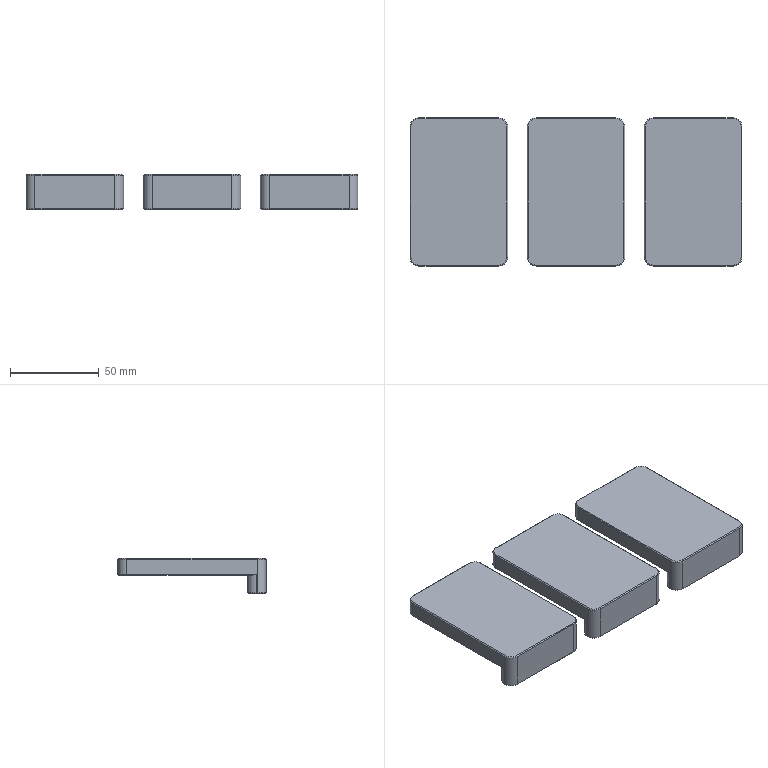NC program | NX | posted with a generic post | part box 187 x 83.5 x 20 mm
Lines 21 to 832 of 5666:
(ZLEVEL_PROFILE_COPY_1 , TOOL : D10)
N40 T15 M6
N42 G54
N44 G17 G0 G90 X-93.244 Y-45.694 S9500 M3
N46 G43 Z30. H15
N48 Z1.5
N50 G94 G1 X-94.903 Y-44.6 Z1.396 F1000.
N52 X-96.35 Y-43.153 Z1.289
N54 X-97.477 Y-41.444 Z1.181
N56 X-98.237 Y-39.543 Z1.074
N58 X-98.6 Y-37.529 Z0.967
N60 Y0. Z-1.
N62 Y36.75 F3500.
N64 G2 X-88.5 Y46.85 R10.1
N66 G1 X-43.5
N68 G2 X-33.4 Y36.75 R10.1
N70 G1 Y-36.75
N72 G2 X-43.5 Y-46.85 R10.1
N74 G1 X-88.5
N76 G2 X-98.6 Y-36.75 R10.1
N78 G1 Y0.
N80 Y36.75 Z-1.122
N82 X-98.574 Y37.471 Z-1.125
N84 X-98.497 Y38.187 Z-1.127
N86 X-98.369 Y38.897 Z-1.13
N88 X-98.191 Y39.595 Z-1.132
N90 X-97.963 Y40.28 Z-1.134
N92 X-97.687 Y40.946 Z-1.137
N94 X-97.365 Y41.59 Z-1.139
N96 X-96.997 Y42.21 Z-1.142
N98 X-96.585 Y42.803 Z-1.144
N100 X-96.133 Y43.364 Z-1.146
N102 X-95.642 Y43.892 Z-1.149
N104 X-95.114 Y44.383 Z-1.151
N106 X-94.553 Y44.835 Z-1.154
N108 X-93.96 Y45.247 Z-1.156
N110 X-93.34 Y45.615 Z-1.158
N112 X-92.696 Y45.937 Z-1.161
N114 X-92.03 Y46.213 Z-1.163
N116 X-91.345 Y46.441 Z-1.166
N118 X-90.647 Y46.619 Z-1.168
N120 X-89.937 Y46.747 Z-1.17
N122 X-89.221 Y46.824 Z-1.173
N124 X-88.5 Y46.85 Z-1.175
N126 X-43.5 Z-1.325
N128 X-42.779 Y46.824 Z-1.327
N130 X-42.063 Y46.747 Z-1.33
N132 X-41.353 Y46.619 Z-1.332
N134 X-40.655 Y46.441 Z-1.334
N136 X-39.97 Y46.213 Z-1.337
N138 X-39.304 Y45.937 Z-1.339
N140 X-38.66 Y45.615 Z-1.342
N142 X-38.04 Y45.247 Z-1.344
N144 X-37.447 Y44.835 Z-1.346
N146 X-36.886 Y44.383 Z-1.349
N148 X-36.358 Y43.892 Z-1.351
N150 X-35.867 Y43.364 Z-1.354
N152 X-35.415 Y42.803 Z-1.356
N154 X-35.003 Y42.21 Z-1.358
N156 X-34.635 Y41.59 Z-1.361
N158 X-34.313 Y40.946 Z-1.363
N160 X-34.037 Y40.28 Z-1.366
N162 X-33.809 Y39.595 Z-1.368
N164 X-33.631 Y38.897 Z-1.37
N166 X-33.503 Y38.187 Z-1.373
N168 X-33.426 Y37.471 Z-1.375
N170 X-33.4 Y36.75 Z-1.378
N172 Y-36.75 Z-1.622
N174 X-33.426 Y-37.471 Z-1.625
N176 X-33.503 Y-38.187 Z-1.627
N178 X-33.631 Y-38.897 Z-1.63
N180 X-33.809 Y-39.595 Z-1.632
N182 X-34.037 Y-40.28 Z-1.634
N184 X-34.313 Y-40.946 Z-1.637
N186 X-34.635 Y-41.59 Z-1.639
N188 X-35.003 Y-42.21 Z-1.642
N190 X-35.415 Y-42.803 Z-1.644
N192 X-35.867 Y-43.364 Z-1.646
N194 X-36.358 Y-43.892 Z-1.649
N196 X-36.886 Y-44.383 Z-1.651
N198 X-37.447 Y-44.835 Z-1.654
N200 X-38.04 Y-45.247 Z-1.656
N202 X-38.66 Y-45.615 Z-1.658
N204 X-39.304 Y-45.937 Z-1.661
N206 X-39.97 Y-46.213 Z-1.663
N208 X-40.655 Y-46.441 Z-1.666
N210 X-41.353 Y-46.619 Z-1.668
N212 X-42.063 Y-46.747 Z-1.67
N214 X-42.779 Y-46.824 Z-1.673
N216 X-43.5 Y-46.85 Z-1.675
N218 X-88.5 Z-1.825
N220 X-89.221 Y-46.824 Z-1.827
N222 X-89.937 Y-46.747 Z-1.83
N224 X-90.647 Y-46.619 Z-1.832
N226 X-91.345 Y-46.441 Z-1.834
N228 X-92.03 Y-46.213 Z-1.837
N230 X-92.696 Y-45.937 Z-1.839
N232 X-93.34 Y-45.615 Z-1.842
N234 X-93.96 Y-45.247 Z-1.844
N236 X-94.553 Y-44.835 Z-1.846
N238 X-95.114 Y-44.383 Z-1.849
N240 X-95.642 Y-43.892 Z-1.851
N242 X-96.133 Y-43.364 Z-1.854
N244 X-96.585 Y-42.803 Z-1.856
N246 X-96.997 Y-42.21 Z-1.858
N248 X-97.365 Y-41.59 Z-1.861
N250 X-97.687 Y-40.946 Z-1.863
N252 X-97.963 Y-40.28 Z-1.866
N254 X-98.191 Y-39.595 Z-1.868
N256 X-98.369 Y-38.897 Z-1.87
N258 X-98.497 Y-38.187 Z-1.873
N260 X-98.574 Y-37.471 Z-1.875
N262 X-98.6 Y-36.75 Z-1.878
N264 Y0. Z-2.
N266 Y36.75 Z-2.122
N268 X-98.574 Y37.471 Z-2.125
N270 X-98.497 Y38.187 Z-2.127
N272 X-98.369 Y38.897 Z-2.13
N274 X-98.191 Y39.595 Z-2.132
N276 X-97.963 Y40.28 Z-2.134
N278 X-97.687 Y40.946 Z-2.137
N280 X-97.365 Y41.59 Z-2.139
N282 X-96.997 Y42.21 Z-2.142
N284 X-96.585 Y42.803 Z-2.144
N286 X-96.133 Y43.364 Z-2.146
N288 X-95.642 Y43.892 Z-2.149
N290 X-95.114 Y44.383 Z-2.151
N292 X-94.553 Y44.835 Z-2.154
N294 X-93.96 Y45.247 Z-2.156
N296 X-93.34 Y45.615 Z-2.158
N298 X-92.696 Y45.937 Z-2.161
N300 X-92.03 Y46.213 Z-2.163
N302 X-91.345 Y46.441 Z-2.166
N304 X-90.647 Y46.619 Z-2.168
N306 X-89.937 Y46.747 Z-2.17
N308 X-89.221 Y46.824 Z-2.173
N310 X-88.5 Y46.85 Z-2.175
N312 X-43.5 Z-2.325
N314 X-42.779 Y46.824 Z-2.327
N316 X-42.063 Y46.747 Z-2.33
N318 X-41.353 Y46.619 Z-2.332
N320 X-40.655 Y46.441 Z-2.334
N322 X-39.97 Y46.213 Z-2.337
N324 X-39.304 Y45.937 Z-2.339
N326 X-38.66 Y45.615 Z-2.342
N328 X-38.04 Y45.247 Z-2.344
N330 X-37.447 Y44.835 Z-2.346
N332 X-36.886 Y44.383 Z-2.349
N334 X-36.358 Y43.892 Z-2.351
N336 X-35.867 Y43.364 Z-2.354
N338 X-35.415 Y42.803 Z-2.356
N340 X-35.003 Y42.21 Z-2.358
N342 X-34.635 Y41.59 Z-2.361
N344 X-34.313 Y40.946 Z-2.363
N346 X-34.037 Y40.28 Z-2.366
N348 X-33.809 Y39.595 Z-2.368
N350 X-33.631 Y38.897 Z-2.37
N352 X-33.503 Y38.187 Z-2.373
N354 X-33.426 Y37.471 Z-2.375
N356 X-33.4 Y36.75 Z-2.378
N358 Y-36.75 Z-2.622
N360 X-33.426 Y-37.471 Z-2.625
N362 X-33.503 Y-38.187 Z-2.627
N364 X-33.631 Y-38.897 Z-2.63
N366 X-33.809 Y-39.595 Z-2.632
N368 X-34.037 Y-40.28 Z-2.634
N370 X-34.313 Y-40.946 Z-2.637
N372 X-34.635 Y-41.59 Z-2.639
N374 X-35.003 Y-42.21 Z-2.642
N376 X-35.415 Y-42.803 Z-2.644
N378 X-35.867 Y-43.364 Z-2.646
N380 X-36.358 Y-43.892 Z-2.649
N382 X-36.886 Y-44.383 Z-2.651
N384 X-37.447 Y-44.835 Z-2.654
N386 X-38.04 Y-45.247 Z-2.656
N388 X-38.66 Y-45.615 Z-2.658
N390 X-39.304 Y-45.937 Z-2.661
N392 X-39.97 Y-46.213 Z-2.663
N394 X-40.655 Y-46.441 Z-2.666
N396 X-41.353 Y-46.619 Z-2.668
N398 X-42.063 Y-46.747 Z-2.67
N400 X-42.779 Y-46.824 Z-2.673
N402 X-43.5 Y-46.85 Z-2.675
N404 X-88.5 Z-2.825
N406 X-89.221 Y-46.824 Z-2.827
N408 X-89.937 Y-46.747 Z-2.83
N410 X-90.647 Y-46.619 Z-2.832
N412 X-91.345 Y-46.441 Z-2.834
N414 X-92.03 Y-46.213 Z-2.837
N416 X-92.696 Y-45.937 Z-2.839
N418 X-93.34 Y-45.615 Z-2.842
N420 X-93.96 Y-45.247 Z-2.844
N422 X-94.553 Y-44.835 Z-2.846
N424 X-95.114 Y-44.383 Z-2.849
N426 X-95.642 Y-43.892 Z-2.851
N428 X-96.133 Y-43.364 Z-2.854
N430 X-96.585 Y-42.803 Z-2.856
N432 X-96.997 Y-42.21 Z-2.858
N434 X-97.365 Y-41.59 Z-2.861
N436 X-97.687 Y-40.946 Z-2.863
N438 X-97.963 Y-40.28 Z-2.866
N440 X-98.191 Y-39.595 Z-2.868
N442 X-98.369 Y-38.897 Z-2.87
N444 X-98.497 Y-38.187 Z-2.873
N446 X-98.574 Y-37.471 Z-2.875
N448 X-98.6 Y-36.75 Z-2.878
N450 Y0. Z-3.
N452 Y36.75 Z-3.122
N454 X-98.574 Y37.471 Z-3.125
N456 X-98.497 Y38.187 Z-3.127
N458 X-98.369 Y38.897 Z-3.13
N460 X-98.191 Y39.595 Z-3.132
N462 X-97.963 Y40.28 Z-3.134
N464 X-97.687 Y40.946 Z-3.137
N466 X-97.365 Y41.59 Z-3.139
N468 X-96.997 Y42.21 Z-3.142
N470 X-96.585 Y42.803 Z-3.144
N472 X-96.133 Y43.364 Z-3.146
N474 X-95.642 Y43.892 Z-3.149
N476 X-95.114 Y44.383 Z-3.151
N478 X-94.553 Y44.835 Z-3.154
N480 X-93.96 Y45.247 Z-3.156
N482 X-93.34 Y45.615 Z-3.158
N484 X-92.696 Y45.937 Z-3.161
N486 X-92.03 Y46.213 Z-3.163
N488 X-91.345 Y46.441 Z-3.166
N490 X-90.647 Y46.619 Z-3.168
N492 X-89.937 Y46.747 Z-3.17
N494 X-89.221 Y46.824 Z-3.173
N496 X-88.5 Y46.85 Z-3.175
N498 X-43.5 Z-3.325
N500 X-42.779 Y46.824 Z-3.327
N502 X-42.063 Y46.747 Z-3.33
N504 X-41.353 Y46.619 Z-3.332
N506 X-40.655 Y46.441 Z-3.334
N508 X-39.97 Y46.213 Z-3.337
N510 X-39.304 Y45.937 Z-3.339
N512 X-38.66 Y45.615 Z-3.342
N514 X-38.04 Y45.247 Z-3.344
N516 X-37.447 Y44.835 Z-3.346
N518 X-36.886 Y44.383 Z-3.349
N520 X-36.358 Y43.892 Z-3.351
N522 X-35.867 Y43.364 Z-3.354
N524 X-35.415 Y42.803 Z-3.356
N526 X-35.003 Y42.21 Z-3.358
N528 X-34.635 Y41.59 Z-3.361
N530 X-34.313 Y40.946 Z-3.363
N532 X-34.037 Y40.28 Z-3.366
N534 X-33.809 Y39.595 Z-3.368
N536 X-33.631 Y38.897 Z-3.37
N538 X-33.503 Y38.187 Z-3.373
N540 X-33.426 Y37.471 Z-3.375
N542 X-33.4 Y36.75 Z-3.378
N544 Y-36.75 Z-3.622
N546 X-33.426 Y-37.471 Z-3.625
N548 X-33.503 Y-38.187 Z-3.627
N550 X-33.631 Y-38.897 Z-3.63
N552 X-33.809 Y-39.595 Z-3.632
N554 X-34.037 Y-40.28 Z-3.634
N556 X-34.313 Y-40.946 Z-3.637
N558 X-34.635 Y-41.59 Z-3.639
N560 X-35.003 Y-42.21 Z-3.642
N562 X-35.415 Y-42.803 Z-3.644
N564 X-35.867 Y-43.364 Z-3.646
N566 X-36.358 Y-43.892 Z-3.649
N568 X-36.886 Y-44.383 Z-3.651
N570 X-37.447 Y-44.835 Z-3.654
N572 X-38.04 Y-45.247 Z-3.656
N574 X-38.66 Y-45.615 Z-3.658
N576 X-39.304 Y-45.937 Z-3.661
N578 X-39.97 Y-46.213 Z-3.663
N580 X-40.655 Y-46.441 Z-3.666
N582 X-41.353 Y-46.619 Z-3.668
N584 X-42.063 Y-46.747 Z-3.67
N586 X-42.779 Y-46.824 Z-3.673
N588 X-43.5 Y-46.85 Z-3.675
N590 X-88.5 Z-3.825
N592 X-89.221 Y-46.824 Z-3.827
N594 X-89.937 Y-46.747 Z-3.83
N596 X-90.647 Y-46.619 Z-3.832
N598 X-91.345 Y-46.441 Z-3.834
N600 X-92.03 Y-46.213 Z-3.837
N602 X-92.696 Y-45.937 Z-3.839
N604 X-93.34 Y-45.615 Z-3.842
N606 X-93.96 Y-45.247 Z-3.844
N608 X-94.553 Y-44.835 Z-3.846
N610 X-95.114 Y-44.383 Z-3.849
N612 X-95.642 Y-43.892 Z-3.851
N614 X-96.133 Y-43.364 Z-3.854
N616 X-96.585 Y-42.803 Z-3.856
N618 X-96.997 Y-42.21 Z-3.858
N620 X-97.365 Y-41.59 Z-3.861
N622 X-97.687 Y-40.946 Z-3.863
N624 X-97.963 Y-40.28 Z-3.866
N626 X-98.191 Y-39.595 Z-3.868
N628 X-98.369 Y-38.897 Z-3.87
N630 X-98.497 Y-38.187 Z-3.873
N632 X-98.574 Y-37.471 Z-3.875
N634 X-98.6 Y-36.75 Z-3.878
N636 Y0. Z-4.
N638 Y36.75 Z-4.122
N640 X-98.574 Y37.471 Z-4.125
N642 X-98.497 Y38.187 Z-4.127
N644 X-98.369 Y38.897 Z-4.13
N646 X-98.191 Y39.595 Z-4.132
N648 X-97.963 Y40.28 Z-4.134
N650 X-97.687 Y40.946 Z-4.137
N652 X-97.365 Y41.59 Z-4.139
N654 X-96.997 Y42.21 Z-4.142
N656 X-96.585 Y42.803 Z-4.144
N658 X-96.133 Y43.364 Z-4.146
N660 X-95.642 Y43.892 Z-4.149
N662 X-95.114 Y44.383 Z-4.151
N664 X-94.553 Y44.835 Z-4.154
N666 X-93.96 Y45.247 Z-4.156
N668 X-93.34 Y45.615 Z-4.158
N670 X-92.696 Y45.937 Z-4.161
N672 X-92.03 Y46.213 Z-4.163
N674 X-91.345 Y46.441 Z-4.166
N676 X-90.647 Y46.619 Z-4.168
N678 X-89.937 Y46.747 Z-4.17
N680 X-89.221 Y46.824 Z-4.173
N682 X-88.5 Y46.85 Z-4.175
N684 X-43.5 Z-4.325
N686 X-42.779 Y46.824 Z-4.327
N688 X-42.063 Y46.747 Z-4.33
N690 X-41.353 Y46.619 Z-4.332
N692 X-40.655 Y46.441 Z-4.334
N694 X-39.97 Y46.213 Z-4.337
N696 X-39.304 Y45.937 Z-4.339
N698 X-38.66 Y45.615 Z-4.342
N700 X-38.04 Y45.247 Z-4.344
N702 X-37.447 Y44.835 Z-4.346
N704 X-36.886 Y44.383 Z-4.349
N706 X-36.358 Y43.892 Z-4.351
N708 X-35.867 Y43.364 Z-4.354
N710 X-35.415 Y42.803 Z-4.356
N712 X-35.003 Y42.21 Z-4.358
N714 X-34.635 Y41.59 Z-4.361
N716 X-34.313 Y40.946 Z-4.363
N718 X-34.037 Y40.28 Z-4.366
N720 X-33.809 Y39.595 Z-4.368
N722 X-33.631 Y38.897 Z-4.37
N724 X-33.503 Y38.187 Z-4.373
N726 X-33.426 Y37.471 Z-4.375
N728 X-33.4 Y36.75 Z-4.378
N730 Y-36.75 Z-4.622
N732 X-33.426 Y-37.471 Z-4.625
N734 X-33.503 Y-38.187 Z-4.627
N736 X-33.631 Y-38.897 Z-4.63
N738 X-33.809 Y-39.595 Z-4.632
N740 X-34.037 Y-40.28 Z-4.634
N742 X-34.313 Y-40.946 Z-4.637
N744 X-34.635 Y-41.59 Z-4.639
N746 X-35.003 Y-42.21 Z-4.642
N748 X-35.415 Y-42.803 Z-4.644
N750 X-35.867 Y-43.364 Z-4.646
N752 X-36.358 Y-43.892 Z-4.649
N754 X-36.886 Y-44.383 Z-4.651
N756 X-37.447 Y-44.835 Z-4.654
N758 X-38.04 Y-45.247 Z-4.656
N760 X-38.66 Y-45.615 Z-4.658
N762 X-39.304 Y-45.937 Z-4.661
N764 X-39.97 Y-46.213 Z-4.663
N766 X-40.655 Y-46.441 Z-4.666
N768 X-41.353 Y-46.619 Z-4.668
N770 X-42.063 Y-46.747 Z-4.67
N772 X-42.779 Y-46.824 Z-4.673
N774 X-43.5 Y-46.85 Z-4.675
N776 X-88.5 Z-4.825
N778 X-89.221 Y-46.824 Z-4.827
N780 X-89.937 Y-46.747 Z-4.83
N782 X-90.647 Y-46.619 Z-4.832
N784 X-91.345 Y-46.441 Z-4.834
N786 X-92.03 Y-46.213 Z-4.837
N788 X-92.696 Y-45.937 Z-4.839
N790 X-93.34 Y-45.615 Z-4.842
N792 X-93.96 Y-45.247 Z-4.844
N794 X-94.553 Y-44.835 Z-4.846
N796 X-95.114 Y-44.383 Z-4.849
N798 X-95.642 Y-43.892 Z-4.851
N800 X-96.133 Y-43.364 Z-4.854
N802 X-96.585 Y-42.803 Z-4.856
N804 X-96.997 Y-42.21 Z-4.858
N806 X-97.365 Y-41.59 Z-4.861
N808 X-97.687 Y-40.946 Z-4.863
N810 X-97.963 Y-40.28 Z-4.866
N812 X-98.191 Y-39.595 Z-4.868
N814 X-98.369 Y-38.897 Z-4.87
N816 X-98.497 Y-38.187 Z-4.873
N818 X-98.574 Y-37.471 Z-4.875
N820 X-98.6 Y-36.75 Z-4.878
N822 Y0. Z-5.
N824 Y36.75 Z-5.122
N826 X-98.574 Y37.471 Z-5.125
N828 X-98.497 Y38.187 Z-5.127
N830 X-98.369 Y38.897 Z-5.13
N832 X-98.191 Y39.595 Z-5.132
N834 X-97.963 Y40.28 Z-5.134
N836 X-97.687 Y40.946 Z-5.137
N838 X-97.365 Y41.59 Z-5.139
N840 X-96.997 Y42.21 Z-5.142
N842 X-96.585 Y42.803 Z-5.144
N844 X-96.133 Y43.364 Z-5.146
N846 X-95.642 Y43.892 Z-5.149
N848 X-95.114 Y44.383 Z-5.151
N850 X-94.553 Y44.835 Z-5.154
N852 X-93.96 Y45.247 Z-5.156
N854 X-93.34 Y45.615 Z-5.158
N856 X-92.696 Y45.937 Z-5.161
N858 X-92.03 Y46.213 Z-5.163
N860 X-91.345 Y46.441 Z-5.166
N862 X-90.647 Y46.619 Z-5.168
N864 X-89.937 Y46.747 Z-5.17
N866 X-89.221 Y46.824 Z-5.173
N868 X-88.5 Y46.85 Z-5.175
N870 X-43.5 Z-5.325
N872 X-42.779 Y46.824 Z-5.327
N874 X-42.063 Y46.747 Z-5.33
N876 X-41.353 Y46.619 Z-5.332
N878 X-40.655 Y46.441 Z-5.334
N880 X-39.97 Y46.213 Z-5.337
N882 X-39.304 Y45.937 Z-5.339
N884 X-38.66 Y45.615 Z-5.342
N886 X-38.04 Y45.247 Z-5.344
N888 X-37.447 Y44.835 Z-5.346
N890 X-36.886 Y44.383 Z-5.349
N892 X-36.358 Y43.892 Z-5.351
N894 X-35.867 Y43.364 Z-5.354
N896 X-35.415 Y42.803 Z-5.356
N898 X-35.003 Y42.21 Z-5.358
N900 X-34.635 Y41.59 Z-5.361
N902 X-34.313 Y40.946 Z-5.363
N904 X-34.037 Y40.28 Z-5.366
N906 X-33.809 Y39.595 Z-5.368
N908 X-33.631 Y38.897 Z-5.37
N910 X-33.503 Y38.187 Z-5.373
N912 X-33.426 Y37.471 Z-5.375
N914 X-33.4 Y36.75 Z-5.378
N916 Y-36.75 Z-5.622
N918 X-33.426 Y-37.471 Z-5.625
N920 X-33.503 Y-38.187 Z-5.627
N922 X-33.631 Y-38.897 Z-5.63
N924 X-33.809 Y-39.595 Z-5.632
N926 X-34.037 Y-40.28 Z-5.634
N928 X-34.313 Y-40.946 Z-5.637
N930 X-34.635 Y-41.59 Z-5.639
N932 X-35.003 Y-42.21 Z-5.642
N934 X-35.415 Y-42.803 Z-5.644
N936 X-35.867 Y-43.364 Z-5.646
N938 X-36.358 Y-43.892 Z-5.649
N940 X-36.886 Y-44.383 Z-5.651
N942 X-37.447 Y-44.835 Z-5.654
N944 X-38.04 Y-45.247 Z-5.656
N946 X-38.66 Y-45.615 Z-5.658
N948 X-39.304 Y-45.937 Z-5.661
N950 X-39.97 Y-46.213 Z-5.663
N952 X-40.655 Y-46.441 Z-5.666
N954 X-41.353 Y-46.619 Z-5.668
N956 X-42.063 Y-46.747 Z-5.67
N958 X-42.779 Y-46.824 Z-5.673
N960 X-43.5 Y-46.85 Z-5.675
N962 X-88.5 Z-5.825
N964 X-89.221 Y-46.824 Z-5.827
N966 X-89.937 Y-46.747 Z-5.83
N968 X-90.647 Y-46.619 Z-5.832
N970 X-91.345 Y-46.441 Z-5.834
N972 X-92.03 Y-46.213 Z-5.837
N974 X-92.696 Y-45.937 Z-5.839
N976 X-93.34 Y-45.615 Z-5.842
N978 X-93.96 Y-45.247 Z-5.844
N980 X-94.553 Y-44.835 Z-5.846
N982 X-95.114 Y-44.383 Z-5.849
N984 X-95.642 Y-43.892 Z-5.851
N986 X-96.133 Y-43.364 Z-5.854
N988 X-96.585 Y-42.803 Z-5.856
N990 X-96.997 Y-42.21 Z-5.858
N992 X-97.365 Y-41.59 Z-5.861
N994 X-97.687 Y-40.946 Z-5.863
N996 X-97.963 Y-40.28 Z-5.866
N998 X-98.191 Y-39.595 Z-5.868
N1000 X-98.369 Y-38.897 Z-5.87
N1002 X-98.497 Y-38.187 Z-5.873
N1004 X-98.574 Y-37.471 Z-5.875
N1006 X-98.6 Y-36.75 Z-5.878
N1008 Y0. Z-6.
N1010 Y36.75 Z-6.122
N1012 X-98.574 Y37.471 Z-6.125
N1014 X-98.497 Y38.187 Z-6.127
N1016 X-98.369 Y38.897 Z-6.13
N1018 X-98.191 Y39.595 Z-6.132
N1020 X-97.963 Y40.28 Z-6.134
N1022 X-97.687 Y40.946 Z-6.137
N1024 X-97.365 Y41.59 Z-6.139
N1026 X-96.997 Y42.21 Z-6.142
N1028 X-96.585 Y42.803 Z-6.144
N1030 X-96.133 Y43.364 Z-6.146
N1032 X-95.642 Y43.892 Z-6.149
N1034 X-95.114 Y44.383 Z-6.151
N1036 X-94.553 Y44.835 Z-6.154
N1038 X-93.96 Y45.247 Z-6.156
N1040 X-93.34 Y45.615 Z-6.158
N1042 X-92.696 Y45.937 Z-6.161
N1044 X-92.03 Y46.213 Z-6.163
N1046 X-91.345 Y46.441 Z-6.166
N1048 X-90.647 Y46.619 Z-6.168
N1050 X-89.937 Y46.747 Z-6.17
N1052 X-89.221 Y46.824 Z-6.173
N1054 X-88.5 Y46.85 Z-6.175
N1056 X-43.5 Z-6.325
N1058 X-42.779 Y46.824 Z-6.327
N1060 X-42.063 Y46.747 Z-6.33
N1062 X-41.353 Y46.619 Z-6.332
N1064 X-40.655 Y46.441 Z-6.334
N1066 X-39.97 Y46.213 Z-6.337
N1068 X-39.304 Y45.937 Z-6.339
N1070 X-38.66 Y45.615 Z-6.342
N1072 X-38.04 Y45.247 Z-6.344
N1074 X-37.447 Y44.835 Z-6.346
N1076 X-36.886 Y44.383 Z-6.349
N1078 X-36.358 Y43.892 Z-6.351
N1080 X-35.867 Y43.364 Z-6.354
N1082 X-35.415 Y42.803 Z-6.356
N1084 X-35.003 Y42.21 Z-6.358
N1086 X-34.635 Y41.59 Z-6.361
N1088 X-34.313 Y40.946 Z-6.363
N1090 X-34.037 Y40.28 Z-6.366
N1092 X-33.809 Y39.595 Z-6.368
N1094 X-33.631 Y38.897 Z-6.37
N1096 X-33.503 Y38.187 Z-6.373
N1098 X-33.426 Y37.471 Z-6.375
N1100 X-33.4 Y36.75 Z-6.378
N1102 Y-36.75 Z-6.622
N1104 X-33.426 Y-37.471 Z-6.625
N1106 X-33.503 Y-38.187 Z-6.627
N1108 X-33.631 Y-38.897 Z-6.63
N1110 X-33.809 Y-39.595 Z-6.632
N1112 X-34.037 Y-40.28 Z-6.634
N1114 X-34.313 Y-40.946 Z-6.637
N1116 X-34.635 Y-41.59 Z-6.639
N1118 X-35.003 Y-42.21 Z-6.642
N1120 X-35.415 Y-42.803 Z-6.644
N1122 X-35.867 Y-43.364 Z-6.646
N1124 X-36.358 Y-43.892 Z-6.649
N1126 X-36.886 Y-44.383 Z-6.651
N1128 X-37.447 Y-44.835 Z-6.654
N1130 X-38.04 Y-45.247 Z-6.656
N1132 X-38.66 Y-45.615 Z-6.658
N1134 X-39.304 Y-45.937 Z-6.661
N1136 X-39.97 Y-46.213 Z-6.663
N1138 X-40.655 Y-46.441 Z-6.666
N1140 X-41.353 Y-46.619 Z-6.668
N1142 X-42.063 Y-46.747 Z-6.67
N1144 X-42.779 Y-46.824 Z-6.673
N1146 X-43.5 Y-46.85 Z-6.675
N1148 X-88.5 Z-6.825
N1150 X-89.221 Y-46.824 Z-6.827
N1152 X-89.937 Y-46.747 Z-6.83
N1154 X-90.647 Y-46.619 Z-6.832
N1156 X-91.345 Y-46.441 Z-6.834
N1158 X-92.03 Y-46.213 Z-6.837
N1160 X-92.696 Y-45.937 Z-6.839
N1162 X-93.34 Y-45.615 Z-6.842
N1164 X-93.96 Y-45.247 Z-6.844
N1166 X-94.553 Y-44.835 Z-6.846
N1168 X-95.114 Y-44.383 Z-6.849
N1170 X-95.642 Y-43.892 Z-6.851
N1172 X-96.133 Y-43.364 Z-6.854
N1174 X-96.585 Y-42.803 Z-6.856
N1176 X-96.997 Y-42.21 Z-6.858
N1178 X-97.365 Y-41.59 Z-6.861
N1180 X-97.687 Y-40.946 Z-6.863
N1182 X-97.963 Y-40.28 Z-6.866
N1184 X-98.191 Y-39.595 Z-6.868
N1186 X-98.369 Y-38.897 Z-6.87
N1188 X-98.497 Y-38.187 Z-6.873
N1190 X-98.574 Y-37.471 Z-6.875
N1192 X-98.6 Y-36.75 Z-6.878
N1194 Y0. Z-7.
N1196 Y36.75 Z-7.122
N1198 X-98.574 Y37.471 Z-7.125
N1200 X-98.497 Y38.187 Z-7.127
N1202 X-98.369 Y38.897 Z-7.13
N1204 X-98.191 Y39.595 Z-7.132
N1206 X-97.963 Y40.28 Z-7.134
N1208 X-97.687 Y40.946 Z-7.137
N1210 X-97.365 Y41.59 Z-7.139
N1212 X-96.997 Y42.21 Z-7.142
N1214 X-96.585 Y42.803 Z-7.144
N1216 X-96.133 Y43.364 Z-7.146
N1218 X-95.642 Y43.892 Z-7.149
N1220 X-95.114 Y44.383 Z-7.151
N1222 X-94.553 Y44.835 Z-7.154
N1224 X-93.96 Y45.247 Z-7.156
N1226 X-93.34 Y45.615 Z-7.158
N1228 X-92.696 Y45.937 Z-7.161
N1230 X-92.03 Y46.213 Z-7.163
N1232 X-91.345 Y46.441 Z-7.166
N1234 X-90.647 Y46.619 Z-7.168
N1236 X-89.937 Y46.747 Z-7.17
N1238 X-89.221 Y46.824 Z-7.173
N1240 X-88.5 Y46.85 Z-7.175
N1242 X-43.5 Z-7.325
N1244 X-42.779 Y46.824 Z-7.327
N1246 X-42.063 Y46.747 Z-7.33
N1248 X-41.353 Y46.619 Z-7.332
N1250 X-40.655 Y46.441 Z-7.334
N1252 X-39.97 Y46.213 Z-7.337
N1254 X-39.304 Y45.937 Z-7.339
N1256 X-38.66 Y45.615 Z-7.342
N1258 X-38.04 Y45.247 Z-7.344
N1260 X-37.447 Y44.835 Z-7.346
N1262 X-36.886 Y44.383 Z-7.349
N1264 X-36.358 Y43.892 Z-7.351
N1266 X-35.867 Y43.364 Z-7.354
N1268 X-35.415 Y42.803 Z-7.356
N1270 X-35.003 Y42.21 Z-7.358
N1272 X-34.635 Y41.59 Z-7.361
N1274 X-34.313 Y40.946 Z-7.363
N1276 X-34.037 Y40.28 Z-7.366
N1278 X-33.809 Y39.595 Z-7.368
N1280 X-33.631 Y38.897 Z-7.37
N1282 X-33.503 Y38.187 Z-7.373
N1284 X-33.426 Y37.471 Z-7.375
N1286 X-33.4 Y36.75 Z-7.378
N1288 Y-36.75 Z-7.622
N1290 X-33.426 Y-37.471 Z-7.625
N1292 X-33.503 Y-38.187 Z-7.627
N1294 X-33.631 Y-38.897 Z-7.63
N1296 X-33.809 Y-39.595 Z-7.632
N1298 X-34.037 Y-40.28 Z-7.634
N1300 X-34.313 Y-40.946 Z-7.637
N1302 X-34.635 Y-41.59 Z-7.639
N1304 X-35.003 Y-42.21 Z-7.642
N1306 X-35.415 Y-42.803 Z-7.644
N1308 X-35.867 Y-43.364 Z-7.646
N1310 X-36.358 Y-43.892 Z-7.649
N1312 X-36.886 Y-44.383 Z-7.651
N1314 X-37.447 Y-44.835 Z-7.654
N1316 X-38.04 Y-45.247 Z-7.656
N1318 X-38.66 Y-45.615 Z-7.658
N1320 X-39.304 Y-45.937 Z-7.661
N1322 X-39.97 Y-46.213 Z-7.663
N1324 X-40.655 Y-46.441 Z-7.666
N1326 X-41.353 Y-46.619 Z-7.668
N1328 X-42.063 Y-46.747 Z-7.67
N1330 X-42.779 Y-46.824 Z-7.673
N1332 X-43.5 Y-46.85 Z-7.675
N1334 X-88.5 Z-7.825
N1336 X-89.221 Y-46.824 Z-7.827
N1338 X-89.937 Y-46.747 Z-7.83
N1340 X-90.647 Y-46.619 Z-7.832
N1342 X-91.345 Y-46.441 Z-7.834
N1344 X-92.03 Y-46.213 Z-7.837
N1346 X-92.696 Y-45.937 Z-7.839
N1348 X-93.34 Y-45.615 Z-7.842
N1350 X-93.96 Y-45.247 Z-7.844
N1352 X-94.553 Y-44.835 Z-7.846
N1354 X-95.114 Y-44.383 Z-7.849
N1356 X-95.642 Y-43.892 Z-7.851
N1358 X-96.133 Y-43.364 Z-7.854
N1360 X-96.585 Y-42.803 Z-7.856
N1362 X-96.997 Y-42.21 Z-7.858
N1364 X-97.365 Y-41.59 Z-7.861
N1366 X-97.687 Y-40.946 Z-7.863
N1368 X-97.963 Y-40.28 Z-7.866
N1370 X-98.191 Y-39.595 Z-7.868
N1372 X-98.369 Y-38.897 Z-7.87
N1374 X-98.497 Y-38.187 Z-7.873
N1376 X-98.574 Y-37.471 Z-7.875
N1378 X-98.6 Y-36.75 Z-7.878
N1380 Y0. Z-8.
N1382 Y36.75 Z-8.122
N1384 X-98.574 Y37.471 Z-8.125
N1386 X-98.497 Y38.187 Z-8.127
N1388 X-98.369 Y38.897 Z-8.13
N1390 X-98.191 Y39.595 Z-8.132
N1392 X-97.963 Y40.28 Z-8.134
N1394 X-97.687 Y40.946 Z-8.137
N1396 X-97.365 Y41.59 Z-8.139
N1398 X-96.997 Y42.21 Z-8.142
N1400 X-96.585 Y42.803 Z-8.144
N1402 X-96.133 Y43.364 Z-8.146
N1404 X-95.642 Y43.892 Z-8.149
N1406 X-95.114 Y44.383 Z-8.151
N1408 X-94.553 Y44.835 Z-8.154
N1410 X-93.96 Y45.247 Z-8.156
N1412 X-93.34 Y45.615 Z-8.158
N1414 X-92.696 Y45.937 Z-8.161
N1416 X-92.03 Y46.213 Z-8.163
N1418 X-91.345 Y46.441 Z-8.166
N1420 X-90.647 Y46.619 Z-8.168
N1422 X-89.937 Y46.747 Z-8.17
N1424 X-89.221 Y46.824 Z-8.173
N1426 X-88.5 Y46.85 Z-8.175
N1428 X-43.5 Z-8.325
N1430 X-42.779 Y46.824 Z-8.327
N1432 X-42.063 Y46.747 Z-8.33
N1434 X-41.353 Y46.619 Z-8.332
N1436 X-40.655 Y46.441 Z-8.334
N1438 X-39.97 Y46.213 Z-8.337
N1440 X-39.304 Y45.937 Z-8.339
N1442 X-38.66 Y45.615 Z-8.342
N1444 X-38.04 Y45.247 Z-8.344
N1446 X-37.447 Y44.835 Z-8.346
N1448 X-36.886 Y44.383 Z-8.349
N1450 X-36.358 Y43.892 Z-8.351
N1452 X-35.867 Y43.364 Z-8.354
N1454 X-35.415 Y42.803 Z-8.356
N1456 X-35.003 Y42.21 Z-8.358
N1458 X-34.635 Y41.59 Z-8.361
N1460 X-34.313 Y40.946 Z-8.363
N1462 X-34.037 Y40.28 Z-8.366
N1464 X-33.809 Y39.595 Z-8.368
N1466 X-33.631 Y38.897 Z-8.37
N1468 X-33.503 Y38.187 Z-8.373
N1470 X-33.426 Y37.471 Z-8.375
N1472 X-33.4 Y36.75 Z-8.378
N1474 Y-36.75 Z-8.622
N1476 X-33.426 Y-37.471 Z-8.625
N1478 X-33.503 Y-38.187 Z-8.627
N1480 X-33.631 Y-38.897 Z-8.63
N1482 X-33.809 Y-39.595 Z-8.632
N1484 X-34.037 Y-40.28 Z-8.634
N1486 X-34.313 Y-40.946 Z-8.637
N1488 X-34.635 Y-41.59 Z-8.639
N1490 X-35.003 Y-42.21 Z-8.642
N1492 X-35.415 Y-42.803 Z-8.644
N1494 X-35.867 Y-43.364 Z-8.646
N1496 X-36.358 Y-43.892 Z-8.649
N1498 X-36.886 Y-44.383 Z-8.651
N1500 X-37.447 Y-44.835 Z-8.654
N1502 X-38.04 Y-45.247 Z-8.656
N1504 X-38.66 Y-45.615 Z-8.658
N1506 X-39.304 Y-45.937 Z-8.661
N1508 X-39.97 Y-46.213 Z-8.663
N1510 X-40.655 Y-46.441 Z-8.666
N1512 X-41.353 Y-46.619 Z-8.668
N1514 X-42.063 Y-46.747 Z-8.67
N1516 X-42.779 Y-46.824 Z-8.673
N1518 X-43.5 Y-46.85 Z-8.675
N1520 X-88.5 Z-8.825
N1522 X-89.221 Y-46.824 Z-8.827
N1524 X-89.937 Y-46.747 Z-8.83
N1526 X-90.647 Y-46.619 Z-8.832
N1528 X-91.345 Y-46.441 Z-8.834
N1530 X-92.03 Y-46.213 Z-8.837
N1532 X-92.696 Y-45.937 Z-8.839
N1534 X-93.34 Y-45.615 Z-8.842
N1536 X-93.96 Y-45.247 Z-8.844
N1538 X-94.553 Y-44.835 Z-8.846
N1540 X-95.114 Y-44.383 Z-8.849
N1542 X-95.642 Y-43.892 Z-8.851
N1544 X-96.133 Y-43.364 Z-8.854
N1546 X-96.585 Y-42.803 Z-8.856
N1548 X-96.997 Y-42.21 Z-8.858
N1550 X-97.365 Y-41.59 Z-8.861
N1552 X-97.687 Y-40.946 Z-8.863
N1554 X-97.963 Y-40.28 Z-8.866
N1556 X-98.191 Y-39.595 Z-8.868
N1558 X-98.369 Y-38.897 Z-8.87
N1560 X-98.497 Y-38.187 Z-8.873
N1562 X-98.574 Y-37.471 Z-8.875
N1564 X-98.6 Y-36.75 Z-8.878
N1566 Y0. Z-9.
N1568 Y36.75 Z-9.122
N1570 X-98.574 Y37.471 Z-9.125
N1572 X-98.497 Y38.187 Z-9.127
N1574 X-98.369 Y38.897 Z-9.13
N1576 X-98.191 Y39.595 Z-9.132
N1578 X-97.963 Y40.28 Z-9.134
N1580 X-97.687 Y40.946 Z-9.137
N1582 X-97.365 Y41.59 Z-9.139
N1584 X-96.997 Y42.21 Z-9.142
N1586 X-96.585 Y42.803 Z-9.144
N1588 X-96.133 Y43.364 Z-9.146
N1590 X-95.642 Y43.892 Z-9.149
N1592 X-95.114 Y44.383 Z-9.151
N1594 X-94.553 Y44.835 Z-9.154
N1596 X-93.96 Y45.247 Z-9.156
N1598 X-93.34 Y45.615 Z-9.158
N1600 X-92.696 Y45.937 Z-9.161
N1602 X-92.03 Y46.213 Z-9.163
N1604 X-91.345 Y46.441 Z-9.166
N1606 X-90.647 Y46.619 Z-9.168
N1608 X-89.937 Y46.747 Z-9.17
N1610 X-89.221 Y46.824 Z-9.173
N1612 X-88.5 Y46.85 Z-9.175
N1614 X-43.5 Z-9.325
N1616 X-42.779 Y46.824 Z-9.327
N1618 X-42.063 Y46.747 Z-9.33
N1620 X-41.353 Y46.619 Z-9.332
N1622 X-40.655 Y46.441 Z-9.334
N1624 X-39.97 Y46.213 Z-9.337
N1626 X-39.304 Y45.937 Z-9.339
N1628 X-38.66 Y45.615 Z-9.342
N1630 X-38.04 Y45.247 Z-9.344
N1632 X-37.447 Y44.835 Z-9.346
N1634 X-36.886 Y44.383 Z-9.349
N1636 X-36.358 Y43.892 Z-9.351
N1638 X-35.867 Y43.364 Z-9.354
N1640 X-35.415 Y42.803 Z-9.356
N1642 X-35.003 Y42.21 Z-9.358
N1644 X-34.635 Y41.59 Z-9.361
N1646 X-34.313 Y40.946 Z-9.363
N1648 X-34.037 Y40.28 Z-9.366
N1650 X-33.809 Y39.595 Z-9.368
N1652 X-33.631 Y38.897 Z-9.37
N1654 X-33.503 Y38.187 Z-9.373
N1656 X-33.426 Y37.471 Z-9.375